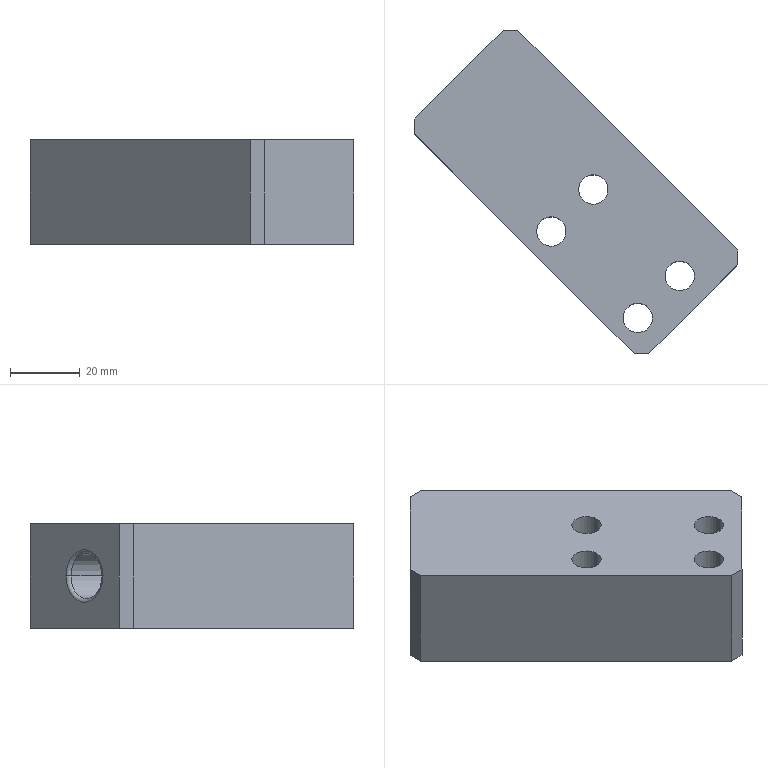Part | STEP file | 1 solid | 23 faces | box 92.631 x 92.631 x 30 mm | volume 108519 mm3 | plane 11 | cylinder 10 | torus 2 | commonest cylinder face diameters 8.4 x8 13 x2